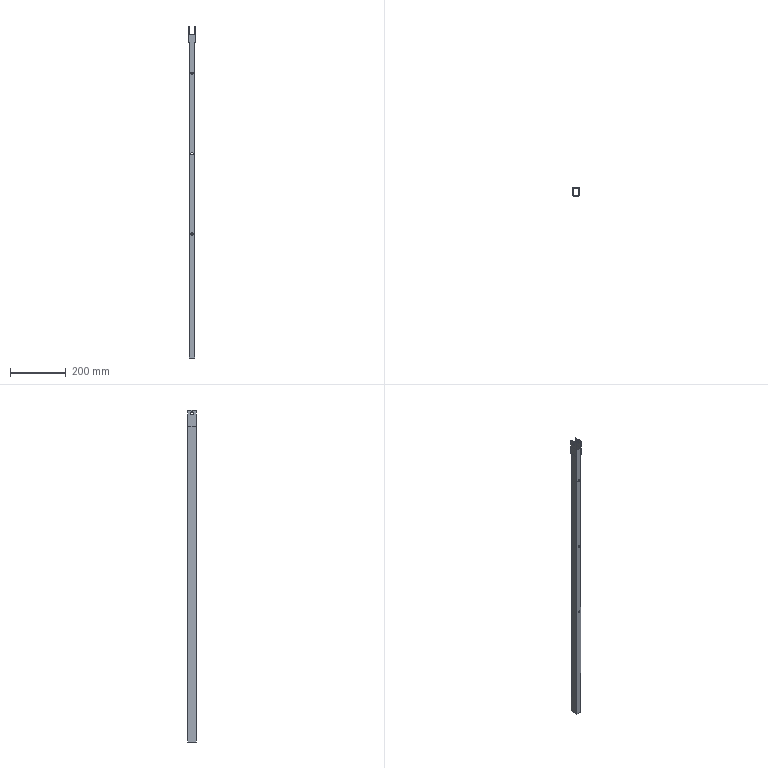Part | SolidWorks | features ICE 4, Extrusion 1, MirrorPattern 1 | 1 solid | 38 faces | box 22 x 30 x 1189 mm | volume 114398 mm3 | cylinder 20 | plane 18 | commonest cylinder face diameters 8 x12 6 x4 10 x4
STEP:
#1=CARTESIAN_POINT('',(10.,-30.,140.));
#2=VERTEX_POINT('',#1);
#3=CARTESIAN_POINT('',(10.,-30.,148.));
#4=VERTEX_POINT('',#3);
#5=CARTESIAN_POINT('',(10.,-30.,144.));
#6=DIRECTION('',(0.,1.,0.));
#7=DIRECTION('',(0.,0.,1.));
#8=AXIS2_PLACEMENT_3D('',#5,#6,#7);
#9=CIRCLE('',#8,4.);
#10=EDGE_CURVE('',#2,#4,#9,.T.);
#11=ORIENTED_EDGE('',*,*,#10,.F.);
#12=CARTESIAN_POINT('',(10.,-29.,140.));
#13=VERTEX_POINT('',#12);
#14=CARTESIAN_POINT('',(10.,-30.,140.));
#15=DIRECTION('',(0.,1.,0.));
#16=VECTOR('',#15,1000.);
#17=LINE('',#14,#16);
#18=EDGE_CURVE('',#2,#13,#17,.T.);
#19=ORIENTED_EDGE('',*,*,#18,.T.);
#20=CARTESIAN_POINT('',(10.,-29.,148.));
#21=VERTEX_POINT('',#20);
#22=CARTESIAN_POINT('',(10.,-29.,144.));
#23=DIRECTION('',(0.,1.,0.));
#24=DIRECTION('',(0.,0.,1.));
#25=AXIS2_PLACEMENT_3D('',#22,#23,#24);
#26=CIRCLE('',#25,4.);
#27=EDGE_CURVE('',#13,#21,#26,.T.);
#28=ORIENTED_EDGE('',*,*,#27,.T.);
#29=CARTESIAN_POINT('',(10.,-30.,148.));
#30=DIRECTION('',(0.,1.,0.));
#31=VECTOR('',#30,1000.);
#32=LINE('',#29,#31);
#33=EDGE_CURVE('',#4,#21,#32,.T.);
#34=ORIENTED_EDGE('',*,*,#33,.F.);
#35=EDGE_LOOP('',(#11,#19,#28,#34));
#36=FACE_OUTER_BOUND('',#35,.T.);
#37=CARTESIAN_POINT('',(10.,-30.,144.));
#38=DIRECTION('',(0.,1.,0.));
#39=DIRECTION('',(0.,0.,1.));
#40=AXIS2_PLACEMENT_3D('',#37,#38,#39);
#41=CYLINDRICAL_SURFACE('',#40,4.);
#42=ADVANCED_FACE('',(#36),#41,.F.);
#43=CARTESIAN_POINT('',(10.,-30.,428.));
#44=VERTEX_POINT('',#43);
#45=CARTESIAN_POINT('',(10.,-30.,436.));
#46=VERTEX_POINT('',#45);
#47=CARTESIAN_POINT('',(10.,-30.,432.));
#48=DIRECTION('',(0.,1.,0.));
#49=DIRECTION('',(0.,0.,1.));
#50=AXIS2_PLACEMENT_3D('',#47,#48,#49);
#51=CIRCLE('',#50,4.);
#52=EDGE_CURVE('',#44,#46,#51,.T.);
#53=ORIENTED_EDGE('',*,*,#52,.F.);
#54=CARTESIAN_POINT('',(10.,-29.,428.));
#55=VERTEX_POINT('',#54);
#56=CARTESIAN_POINT('',(10.,-30.,428.));
#57=DIRECTION('',(0.,1.,0.));
#58=VECTOR('',#57,1000.);
#59=LINE('',#56,#58);
#60=EDGE_CURVE('',#44,#55,#59,.T.);
#61=ORIENTED_EDGE('',*,*,#60,.T.);
#62=CARTESIAN_POINT('',(10.,-29.,436.));
#63=VERTEX_POINT('',#62);
#64=CARTESIAN_POINT('',(10.,-29.,432.));
#65=DIRECTION('',(0.,1.,0.));
#66=DIRECTION('',(0.,0.,1.));
#67=AXIS2_PLACEMENT_3D('',#64,#65,#66);
#68=CIRCLE('',#67,4.);
#69=EDGE_CURVE('',#55,#63,#68,.T.);
#70=ORIENTED_EDGE('',*,*,#69,.T.);
#71=CARTESIAN_POINT('',(10.,-30.,436.));
#72=DIRECTION('',(0.,1.,0.));
#73=VECTOR('',#72,1000.);
#74=LINE('',#71,#73);
#75=EDGE_CURVE('',#46,#63,#74,.T.);
#76=ORIENTED_EDGE('',*,*,#75,.F.);
#77=EDGE_LOOP('',(#53,#61,#70,#76));
#78=FACE_OUTER_BOUND('',#77,.T.);
#79=CARTESIAN_POINT('',(10.,-30.,432.));
#80=DIRECTION('',(0.,1.,0.));
#81=DIRECTION('',(0.,0.,1.));
#82=AXIS2_PLACEMENT_3D('',#79,#80,#81);
#83=CYLINDRICAL_SURFACE('',#82,4.);
#84=ADVANCED_FACE('',(#78),#83,.F.);
#85=CARTESIAN_POINT('',(10.,-30.,716.));
#86=VERTEX_POINT('',#85);
#87=CARTESIAN_POINT('',(10.,-30.,724.));
#88=VERTEX_POINT('',#87);
#89=CARTESIAN_POINT('',(10.,-30.,720.));
#90=DIRECTION('',(0.,1.,0.));
#91=DIRECTION('',(0.,0.,1.));
#92=AXIS2_PLACEMENT_3D('',#89,#90,#91);
#93=CIRCLE('',#92,4.);
#94=EDGE_CURVE('',#86,#88,#93,.T.);
#95=ORIENTED_EDGE('',*,*,#94,.F.);
#96=CARTESIAN_POINT('',(10.,-29.,716.));
#97=VERTEX_POINT('',#96);
#98=CARTESIAN_POINT('',(10.,-30.,716.));
#99=DIRECTION('',(0.,1.,0.));
#100=VECTOR('',#99,1000.);
#101=LINE('',#98,#100);
#102=EDGE_CURVE('',#86,#97,#101,.T.);
#103=ORIENTED_EDGE('',*,*,#102,.T.);
#104=CARTESIAN_POINT('',(10.,-29.,724.));
#105=VERTEX_POINT('',#104);
#106=CARTESIAN_POINT('',(10.,-29.,720.));
#107=DIRECTION('',(0.,1.,0.));
#108=DIRECTION('',(0.,0.,1.));
#109=AXIS2_PLACEMENT_3D('',#106,#107,#108);
#110=CIRCLE('',#109,4.);
#111=EDGE_CURVE('',#97,#105,#110,.T.);
#112=ORIENTED_EDGE('',*,*,#111,.T.);
#113=CARTESIAN_POINT('',(10.,-30.,724.));
#114=DIRECTION('',(0.,1.,0.));
#115=VECTOR('',#114,1000.);
#116=LINE('',#113,#115);
#117=EDGE_CURVE('',#88,#105,#116,.T.);
#118=ORIENTED_EDGE('',*,*,#117,.F.);
#119=EDGE_LOOP('',(#95,#103,#112,#118));
#120=FACE_OUTER_BOUND('',#119,.T.);
#121=CARTESIAN_POINT('',(10.,-30.,720.));
#122=DIRECTION('',(0.,1.,0.));
#123=DIRECTION('',(0.,0.,1.));
#124=AXIS2_PLACEMENT_3D('',#121,#122,#123);
#125=CYLINDRICAL_SURFACE('',#124,4.);
#126=ADVANCED_FACE('',(#120),#125,.F.);
#127=CARTESIAN_POINT('',(10.,-1.,148.));
#128=VERTEX_POINT('',#127);
#129=CARTESIAN_POINT('',(10.,-1.,140.));
#130=VERTEX_POINT('',#129);
#131=CARTESIAN_POINT('',(10.,-1.,144.));
#132=DIRECTION('',(0.,-1.,0.));
#133=DIRECTION('',(0.,0.,-1.));
#134=AXIS2_PLACEMENT_3D('',#131,#132,#133);
#135=CIRCLE('',#134,4.);
#136=EDGE_CURVE('',#128,#130,#135,.T.);
#137=ORIENTED_EDGE('',*,*,#136,.T.);
#138=CARTESIAN_POINT('',(10.,0.,140.));
#139=VERTEX_POINT('',#138);
#140=CARTESIAN_POINT('',(10.,-30.,140.));
#141=DIRECTION('',(0.,1.,0.));
#142=VECTOR('',#141,1000.);
#143=LINE('',#140,#142);
#144=EDGE_CURVE('',#130,#139,#143,.T.);
#145=ORIENTED_EDGE('',*,*,#144,.T.);
#146=CARTESIAN_POINT('',(10.,0.,148.));
#147=VERTEX_POINT('',#146);
#148=CARTESIAN_POINT('',(10.,0.,144.));
#149=DIRECTION('',(0.,1.,0.));
#150=DIRECTION('',(0.,0.,1.));
#151=AXIS2_PLACEMENT_3D('',#148,#149,#150);
#152=CIRCLE('',#151,4.);
#153=EDGE_CURVE('',#139,#147,#152,.T.);
#154=ORIENTED_EDGE('',*,*,#153,.T.);
#155=CARTESIAN_POINT('',(10.,-30.,148.));
#156=DIRECTION('',(0.,1.,0.));
#157=VECTOR('',#156,1000.);
#158=LINE('',#155,#157);
#159=EDGE_CURVE('',#128,#147,#158,.T.);
#160=ORIENTED_EDGE('',*,*,#159,.F.);
#161=EDGE_LOOP('',(#137,#145,#154,#160));
#162=FACE_OUTER_BOUND('',#161,.T.);
#163=CARTESIAN_POINT('',(10.,-30.,144.));
#164=DIRECTION('',(0.,1.,0.));
#165=DIRECTION('',(0.,0.,1.));
#166=AXIS2_PLACEMENT_3D('',#163,#164,#165);
#167=CYLINDRICAL_SURFACE('',#166,4.);
#168=ADVANCED_FACE('',(#162),#167,.F.);
#169=CARTESIAN_POINT('',(10.,-1.,436.));
#170=VERTEX_POINT('',#169);
#171=CARTESIAN_POINT('',(10.,-1.,428.));
#172=VERTEX_POINT('',#171);
#173=CARTESIAN_POINT('',(10.,-1.,432.));
#174=DIRECTION('',(0.,-1.,0.));
#175=DIRECTION('',(0.,0.,-1.));
#176=AXIS2_PLACEMENT_3D('',#173,#174,#175);
#177=CIRCLE('',#176,4.);
#178=EDGE_CURVE('',#170,#172,#177,.T.);
#179=ORIENTED_EDGE('',*,*,#178,.T.);
#180=CARTESIAN_POINT('',(10.,0.,428.));
#181=VERTEX_POINT('',#180);
#182=CARTESIAN_POINT('',(10.,-30.,428.));
#183=DIRECTION('',(0.,1.,0.));
#184=VECTOR('',#183,1000.);
#185=LINE('',#182,#184);
#186=EDGE_CURVE('',#172,#181,#185,.T.);
#187=ORIENTED_EDGE('',*,*,#186,.T.);
#188=CARTESIAN_POINT('',(10.,0.,436.));
#189=VERTEX_POINT('',#188);
#190=CARTESIAN_POINT('',(10.,0.,432.));
#191=DIRECTION('',(0.,1.,0.));
#192=DIRECTION('',(0.,0.,1.));
#193=AXIS2_PLACEMENT_3D('',#190,#191,#192);
#194=CIRCLE('',#193,4.);
#195=EDGE_CURVE('',#181,#189,#194,.T.);
#196=ORIENTED_EDGE('',*,*,#195,.T.);
#197=CARTESIAN_POINT('',(10.,-30.,436.));
#198=DIRECTION('',(0.,1.,0.));
#199=VECTOR('',#198,1000.);
#200=LINE('',#197,#199);
#201=EDGE_CURVE('',#170,#189,#200,.T.);
#202=ORIENTED_EDGE('',*,*,#201,.F.);
#203=EDGE_LOOP('',(#179,#187,#196,#202));
#204=FACE_OUTER_BOUND('',#203,.T.);
#205=CARTESIAN_POINT('',(10.,-30.,432.));
#206=DIRECTION('',(0.,1.,0.));
#207=DIRECTION('',(0.,0.,1.));
#208=AXIS2_PLACEMENT_3D('',#205,#206,#207);
#209=CYLINDRICAL_SURFACE('',#208,4.);
#210=ADVANCED_FACE('',(#204),#209,.F.);
#211=CARTESIAN_POINT('',(10.,-1.,724.));
#212=VERTEX_POINT('',#211);
#213=CARTESIAN_POINT('',(10.,-1.,716.));
#214=VERTEX_POINT('',#213);
#215=CARTESIAN_POINT('',(10.,-1.,720.));
#216=DIRECTION('',(0.,-1.,0.));
#217=DIRECTION('',(0.,0.,-1.));
#218=AXIS2_PLACEMENT_3D('',#215,#216,#217);
#219=CIRCLE('',#218,4.);
#220=EDGE_CURVE('',#212,#214,#219,.T.);
#221=ORIENTED_EDGE('',*,*,#220,.T.);
#222=CARTESIAN_POINT('',(10.,0.,716.));
#223=VERTEX_POINT('',#222);
#224=CARTESIAN_POINT('',(10.,-30.,716.));
#225=DIRECTION('',(0.,1.,0.));
#226=VECTOR('',#225,1000.);
#227=LINE('',#224,#226);
#228=EDGE_CURVE('',#214,#223,#227,.T.);
#229=ORIENTED_EDGE('',*,*,#228,.T.);
#230=CARTESIAN_POINT('',(10.,0.,724.));
#231=VERTEX_POINT('',#230);
#232=CARTESIAN_POINT('',(10.,0.,720.));
#233=DIRECTION('',(0.,1.,0.));
#234=DIRECTION('',(0.,0.,1.));
#235=AXIS2_PLACEMENT_3D('',#232,#233,#234);
#236=CIRCLE('',#235,4.);
#237=EDGE_CURVE('',#223,#231,#236,.T.);
#238=ORIENTED_EDGE('',*,*,#237,.T.);
#239=CARTESIAN_POINT('',(10.,-30.,724.));
#240=DIRECTION('',(0.,1.,0.));
#241=VECTOR('',#240,1000.);
#242=LINE('',#239,#241);
#243=EDGE_CURVE('',#212,#231,#242,.T.);
#244=ORIENTED_EDGE('',*,*,#243,.F.);
#245=EDGE_LOOP('',(#221,#229,#238,#244));
#246=FACE_OUTER_BOUND('',#245,.T.);
#247=CARTESIAN_POINT('',(10.,-30.,720.));
#248=DIRECTION('',(0.,1.,0.));
#249=DIRECTION('',(0.,0.,1.));
#250=AXIS2_PLACEMENT_3D('',#247,#248,#249);
#251=CYLINDRICAL_SURFACE('',#250,4.);
#252=ADVANCED_FACE('',(#246),#251,.F.);
#253=CARTESIAN_POINT('',(-1.,-20.,877.5));
#254=VERTEX_POINT('',#253);
#255=CARTESIAN_POINT('',(-1.,-10.,877.5));
#256=VERTEX_POINT('',#255);
#257=CARTESIAN_POINT('',(-1.,-15.,877.5));
#258=DIRECTION('',(1.,0.,0.));
#259=DIRECTION('',(0.,1.,0.));
#260=AXIS2_PLACEMENT_3D('',#257,#258,#259);
#261=CIRCLE('',#260,5.);
#262=EDGE_CURVE('',#254,#256,#261,.T.);
#263=ORIENTED_EDGE('',*,*,#262,.F.);
#264=CARTESIAN_POINT('',(0.,-20.,877.5));
#265=VERTEX_POINT('',#264);
#266=CARTESIAN_POINT('',(-1.,-20.,877.5));
#267=DIRECTION('',(1.,0.,0.));
#268=VECTOR('',#267,1000.);
#269=LINE('',#266,#268);
#270=EDGE_CURVE('',#254,#265,#269,.T.);
#271=ORIENTED_EDGE('',*,*,#270,.T.);
#272=CARTESIAN_POINT('',(0.,-10.,877.5));
#273=VERTEX_POINT('',#272);
#274=CARTESIAN_POINT('',(0.,-15.,877.5));
#275=DIRECTION('',(-1.,0.,0.));
#276=DIRECTION('',(0.,-1.,0.));
#277=AXIS2_PLACEMENT_3D('',#274,#275,#276);
#278=CIRCLE('',#277,5.);
#279=EDGE_CURVE('',#273,#265,#278,.T.);
#280=ORIENTED_EDGE('',*,*,#279,.F.);
#281=CARTESIAN_POINT('',(-1.,-10.,877.5));
#282=DIRECTION('',(1.,0.,0.));
#283=VECTOR('',#282,1000.);
#284=LINE('',#281,#283);
#285=EDGE_CURVE('',#256,#273,#284,.T.);
#286=ORIENTED_EDGE('',*,*,#285,.F.);
#287=EDGE_LOOP('',(#263,#271,#280,#286));
#288=FACE_OUTER_BOUND('',#287,.T.);
#289=CARTESIAN_POINT('',(-1.,-15.,877.5));
#290=DIRECTION('',(1.,0.,0.));
#291=DIRECTION('',(0.,1.,0.));
#292=AXIS2_PLACEMENT_3D('',#289,#290,#291);
#293=CYLINDRICAL_SURFACE('',#292,5.);
#294=ADVANCED_FACE('',(#288),#293,.F.);
#295=CARTESIAN_POINT('',(20.,-20.,877.5));
#296=VERTEX_POINT('',#295);
#297=CARTESIAN_POINT('',(20.,-10.,877.5));
#298=VERTEX_POINT('',#297);
#299=CARTESIAN_POINT('',(20.,-15.,877.5));
#300=DIRECTION('',(1.,0.,0.));
#301=DIRECTION('',(0.,1.,0.));
#302=AXIS2_PLACEMENT_3D('',#299,#300,#301);
#303=CIRCLE('',#302,5.);
#304=EDGE_CURVE('',#296,#298,#303,.T.);
#305=ORIENTED_EDGE('',*,*,#304,.F.);
#306=CARTESIAN_POINT('',(21.,-20.,877.5));
#307=VERTEX_POINT('',#306);
#308=CARTESIAN_POINT('',(-1.,-20.,877.5));
#309=DIRECTION('',(1.,0.,0.));
#310=VECTOR('',#309,1000.);
#311=LINE('',#308,#310);
#312=EDGE_CURVE('',#296,#307,#311,.T.);
#313=ORIENTED_EDGE('',*,*,#312,.T.);
#314=CARTESIAN_POINT('',(21.,-10.,877.5));
#315=VERTEX_POINT('',#314);
#316=CARTESIAN_POINT('',(21.,-15.,877.5));
#317=DIRECTION('',(1.,0.,0.));
#318=DIRECTION('',(0.,1.,0.));
#319=AXIS2_PLACEMENT_3D('',#316,#317,#318);
#320=CIRCLE('',#319,5.);
#321=EDGE_CURVE('',#307,#315,#320,.T.);
#322=ORIENTED_EDGE('',*,*,#321,.T.);
#323=CARTESIAN_POINT('',(-1.,-10.,877.5));
#324=DIRECTION('',(1.,0.,0.));
#325=VECTOR('',#324,1000.);
#326=LINE('',#323,#325);
#327=EDGE_CURVE('',#298,#315,#326,.T.);
#328=ORIENTED_EDGE('',*,*,#327,.F.);
#329=EDGE_LOOP('',(#305,#313,#322,#328));
#330=FACE_OUTER_BOUND('',#329,.T.);
#331=CARTESIAN_POINT('',(-1.,-15.,877.5));
#332=DIRECTION('',(1.,0.,0.));
#333=DIRECTION('',(0.,1.,0.));
#334=AXIS2_PLACEMENT_3D('',#331,#332,#333);
#335=CYLINDRICAL_SURFACE('',#334,5.);
#336=ADVANCED_FACE('',(#330),#335,.F.);
#337=CARTESIAN_POINT('',(0.,0.,829.));
#338=VERTEX_POINT('',#337);
#339=CARTESIAN_POINT('',(0.,-30.,829.));
#340=VERTEX_POINT('',#339);
#341=CARTESIAN_POINT('',(0.,-30.,829.));
#342=DIRECTION('',(0.,-1.,0.));
#343=VECTOR('',#342,1000.);
#344=LINE('',#341,#343);
#345=EDGE_CURVE('',#338,#340,#344,.T.);
#346=ORIENTED_EDGE('',*,*,#345,.F.);
#347=CARTESIAN_POINT('',(0.,0.,-300.));
#348=VERTEX_POINT('',#347);
#349=CARTESIAN_POINT('',(0.,0.,859.));
#350=DIRECTION('',(0.,0.,-1.));
#351=VECTOR('',#350,1000.);
#352=LINE('',#349,#351);
#353=EDGE_CURVE('',#338,#348,#352,.T.);
#354=ORIENTED_EDGE('',*,*,#353,.T.);
#355=CARTESIAN_POINT('',(0.,-30.,-300.));
#356=VERTEX_POINT('',#355);
#357=CARTESIAN_POINT('',(0.,-30.,-300.));
#358=DIRECTION('',(0.,1.,0.));
#359=VECTOR('',#358,1000.);
#360=LINE('',#357,#359);
#361=EDGE_CURVE('',#356,#348,#360,.T.);
#362=ORIENTED_EDGE('',*,*,#361,.F.);
#363=CARTESIAN_POINT('',(0.,-30.,859.));
#364=DIRECTION('',(0.,0.,-1.));
#365=VECTOR('',#364,1000.);
#366=LINE('',#363,#365);
#367=EDGE_CURVE('',#340,#356,#366,.T.);
#368=ORIENTED_EDGE('',*,*,#367,.F.);
#369=EDGE_LOOP('',(#346,#354,#362,#368));
#370=FACE_OUTER_BOUND('',#369,.T.);
#371=CARTESIAN_POINT('',(0.,0.,859.));
#372=DIRECTION('',(1.,0.,0.));
#373=DIRECTION('',(0.,1.,0.));
#374=AXIS2_PLACEMENT_3D('',#371,#372,#373);
#375=PLANE('',#374);
#376=ADVANCED_FACE('',(#370),#375,.F.);
#377=CARTESIAN_POINT('',(0.,0.,859.));
#378=VERTEX_POINT('',#377);
#379=CARTESIAN_POINT('',(0.,-30.,859.));
#380=VERTEX_POINT('',#379);
#381=CARTESIAN_POINT('',(0.,0.,859.));
#382=DIRECTION('',(0.,-1.,0.));
#383=VECTOR('',#382,1000.);
#384=LINE('',#381,#383);
#385=EDGE_CURVE('',#378,#380,#384,.T.);
#386=ORIENTED_EDGE('',*,*,#385,.T.);
#387=CARTESIAN_POINT('',(20.,-30.,859.));
#388=VERTEX_POINT('',#387);
#389=CARTESIAN_POINT('',(0.,-30.,859.));
#390=DIRECTION('',(1.,0.,0.));
#391=VECTOR('',#390,1000.);
#392=LINE('',#389,#391);
#393=EDGE_CURVE('',#380,#388,#392,.T.);
#394=ORIENTED_EDGE('',*,*,#393,.T.);
#395=CARTESIAN_POINT('',(20.,0.,859.));
#396=VERTEX_POINT('',#395);
#397=CARTESIAN_POINT('',(20.,0.,859.));
#398=DIRECTION('',(0.,1.,0.));
#399=VECTOR('',#398,1000.);
#400=LINE('',#397,#399);
#401=EDGE_CURVE('',#388,#396,#400,.T.);
#402=ORIENTED_EDGE('',*,*,#401,.T.);
#403=CARTESIAN_POINT('',(0.,0.,859.));
#404=DIRECTION('',(-1.,0.,0.));
#405=VECTOR('',#404,1000.);
#406=LINE('',#403,#405);
#407=EDGE_CURVE('',#396,#378,#406,.T.);
#408=ORIENTED_EDGE('',*,*,#407,.T.);
#409=EDGE_LOOP('',(#386,#394,#402,#408));
#410=FACE_OUTER_BOUND('',#409,.T.);
#411=CARTESIAN_POINT('',(1.,-29.,859.));
#412=VERTEX_POINT('',#411);
#413=CARTESIAN_POINT('',(19.,-29.,859.));
#414=VERTEX_POINT('',#413);
#415=CARTESIAN_POINT('',(1.,-29.,859.));
#416=DIRECTION('',(1.,0.,0.));
#417=VECTOR('',#416,1000.);
#418=LINE('',#415,#417);
#419=EDGE_CURVE('',#412,#414,#418,.T.);
#420=ORIENTED_EDGE('',*,*,#419,.F.);
#421=CARTESIAN_POINT('',(1.,-1.,859.));
#422=VERTEX_POINT('',#421);
#423=CARTESIAN_POINT('',(1.,-1.,859.));
#424=DIRECTION('',(0.,-1.,0.));
#425=VECTOR('',#424,1000.);
#426=LINE('',#423,#425);
#427=EDGE_CURVE('',#422,#412,#426,.T.);
#428=ORIENTED_EDGE('',*,*,#427,.F.);
#429=CARTESIAN_POINT('',(19.,-1.,859.));
#430=VERTEX_POINT('',#429);
#431=CARTESIAN_POINT('',(1.,-1.,859.));
#432=DIRECTION('',(-1.,0.,0.));
#433=VECTOR('',#432,1000.);
#434=LINE('',#431,#433);
#435=EDGE_CURVE('',#430,#422,#434,.T.);
#436=ORIENTED_EDGE('',*,*,#435,.F.);
#437=CARTESIAN_POINT('',(19.,-1.,859.));
#438=DIRECTION('',(0.,1.,0.));
#439=VECTOR('',#438,1000.);
#440=LINE('',#437,#439);
#441=EDGE_CURVE('',#414,#430,#440,.T.);
#442=ORIENTED_EDGE('',*,*,#441,.F.);
#443=EDGE_LOOP('',(#420,#428,#436,#442));
#444=FACE_BOUND('',#443,.T.);
#445=CARTESIAN_POINT('',(0.,0.,859.));
#446=DIRECTION('',(0.,0.,1.));
#447=DIRECTION('',(1.,0.,0.));
#448=AXIS2_PLACEMENT_3D('',#445,#446,#447);
#449=PLANE('',#448);
#450=ADVANCED_FACE('',(#410,#444),#449,.T.);
#451=CARTESIAN_POINT('',(10.,-30.,144.));
#452=DIRECTION('',(0.,1.,0.));
#453=DIRECTION('',(0.,0.,1.));
#454=AXIS2_PLACEMENT_3D('',#451,#452,#453);
#455=CIRCLE('',#454,4.);
#456=EDGE_CURVE('',#4,#2,#455,.T.);
#457=ORIENTED_EDGE('',*,*,#456,.T.);
#458=ORIENTED_EDGE('',*,*,#10,.T.);
#459=EDGE_LOOP('',(#457,#458));
#460=FACE_BOUND('',#459,.T.);
#461=CARTESIAN_POINT('',(10.,-30.,432.));
#462=DIRECTION('',(0.,1.,0.));
#463=DIRECTION('',(0.,0.,1.));
#464=AXIS2_PLACEMENT_3D('',#461,#462,#463);
#465=CIRCLE('',#464,4.);
#466=EDGE_CURVE('',#46,#44,#465,.T.);
#467=ORIENTED_EDGE('',*,*,#466,.T.);
#468=ORIENTED_EDGE('',*,*,#52,.T.);
#469=EDGE_LOOP('',(#467,#468));
#470=FACE_BOUND('',#469,.T.);
#471=CARTESIAN_POINT('',(10.,-30.,720.));
#472=DIRECTION('',(0.,1.,0.));
#473=DIRECTION('',(0.,0.,1.));
#474=AXIS2_PLACEMENT_3D('',#471,#472,#473);
#475=CIRCLE('',#474,4.);
#476=EDGE_CURVE('',#88,#86,#475,.T.);
#477=ORIENTED_EDGE('',*,*,#476,.T.);
#478=ORIENTED_EDGE('',*,*,#94,.T.);
#479=EDGE_LOOP('',(#477,#478));
#480=FACE_BOUND('',#479,.T.);
#481=ORIENTED_EDGE('',*,*,#367,.T.);
#482=CARTESIAN_POINT('',(20.,-30.,-300.));
#483=VERTEX_POINT('',#482);
#484=CARTESIAN_POINT('',(20.,-30.,-300.));
#485=DIRECTION('',(-1.,0.,0.));
#486=VECTOR('',#485,1000.);
#487=LINE('',#484,#486);
#488=EDGE_CURVE('',#483,#356,#487,.T.);
#489=ORIENTED_EDGE('',*,*,#488,.F.);
#490=CARTESIAN_POINT('',(20.,-30.,829.));
#491=VERTEX_POINT('',#490);
#492=CARTESIAN_POINT('',(20.,-30.,859.));
#493=DIRECTION('',(0.,0.,-1.));
#494=VECTOR('',#493,1000.);
#495=LINE('',#492,#494);
#496=EDGE_CURVE('',#491,#483,#495,.T.);
#497=ORIENTED_EDGE('',*,*,#496,.F.);
#498=CARTESIAN_POINT('',(21.,-30.,829.));
#499=VERTEX_POINT('',#498);
#500=CARTESIAN_POINT('',(21.,-30.,829.));
#501=DIRECTION('',(-1.,0.,0.));
#502=VECTOR('',#501,1000.);
#503=LINE('',#500,#502);
#504=EDGE_CURVE('',#499,#491,#503,.T.);
#505=ORIENTED_EDGE('',*,*,#504,.F.);
#506=CARTESIAN_POINT('',(21.,-30.,886.));
#507=VERTEX_POINT('',#506);
#508=CARTESIAN_POINT('',(21.,-30.,859.));
#509=DIRECTION('',(0.,0.,1.));
#510=VECTOR('',#509,1000.);
#511=LINE('',#508,#510);
#512=EDGE_CURVE('',#499,#507,#511,.T.);
#513=ORIENTED_EDGE('',*,*,#512,.T.);
#514=CARTESIAN_POINT('',(20.,-30.,886.));
#515=VERTEX_POINT('',#514);
#516=CARTESIAN_POINT('',(21.,-30.,886.));
#517=DIRECTION('',(-1.,0.,0.));
#518=VECTOR('',#517,1000.);
#519=LINE('',#516,#518);
#520=EDGE_CURVE('',#507,#515,#519,.T.);
#521=ORIENTED_EDGE('',*,*,#520,.T.);
#522=CARTESIAN_POINT('',(20.,-30.,829.));
#523=DIRECTION('',(0.,0.,1.));
#524=VECTOR('',#523,1000.);
#525=LINE('',#522,#524);
#526=EDGE_CURVE('',#388,#515,#525,.T.);
#527=ORIENTED_EDGE('',*,*,#526,.F.);
#528=ORIENTED_EDGE('',*,*,#393,.F.);
#529=CARTESIAN_POINT('',(0.,-30.,886.));
#530=VERTEX_POINT('',#529);
#531=CARTESIAN_POINT('',(0.,-30.,859.));
#532=DIRECTION('',(0.,0.,1.));
#533=VECTOR('',#532,1000.);
#534=LINE('',#531,#533);
#535=EDGE_CURVE('',#380,#530,#534,.T.);
#536=ORIENTED_EDGE('',*,*,#535,.T.);
#537=CARTESIAN_POINT('',(-1.,-30.,886.));
#538=VERTEX_POINT('',#537);
#539=CARTESIAN_POINT('',(-1.,-30.,886.));
#540=DIRECTION('',(1.,0.,0.));
#541=VECTOR('',#540,1000.);
#542=LINE('',#539,#541);
#543=EDGE_CURVE('',#538,#530,#542,.T.);
#544=ORIENTED_EDGE('',*,*,#543,.F.);
#545=CARTESIAN_POINT('',(-1.,-30.,829.));
#546=VERTEX_POINT('',#545);
#547=CARTESIAN_POINT('',(-1.,-30.,829.));
#548=DIRECTION('',(0.,0.,1.));
#549=VECTOR('',#548,1000.);
#550=LINE('',#547,#549);
#551=EDGE_CURVE('',#546,#538,#550,.T.);
#552=ORIENTED_EDGE('',*,*,#551,.F.);
#553=CARTESIAN_POINT('',(-1.,-30.,829.));
#554=DIRECTION('',(1.,0.,0.));
#555=VECTOR('',#554,1000.);
#556=LINE('',#553,#555);
#557=EDGE_CURVE('',#546,#340,#556,.T.);
#558=ORIENTED_EDGE('',*,*,#557,.T.);
#559=EDGE_LOOP('',(#481,#489,#497,#505,#513,#521,#527,#528,#536,#544,#552,#558));
#560=FACE_OUTER_BOUND('',#559,.T.);
#561=CARTESIAN_POINT('',(0.,-30.,859.));
#562=DIRECTION('',(0.,1.,0.));
#563=DIRECTION('',(0.,0.,1.));
#564=AXIS2_PLACEMENT_3D('',#561,#562,#563);
#565=PLANE('',#564);
#566=ADVANCED_FACE('',(#460,#470,#480,#560),#565,.F.);
#567=CARTESIAN_POINT('',(20.,0.,829.));
#568=VERTEX_POINT('',#567);
#569=CARTESIAN_POINT('',(20.,0.,-300.));
#570=VERTEX_POINT('',#569);
#571=CARTESIAN_POINT('',(20.,0.,859.));
#572=DIRECTION('',(0.,0.,-1.));
#573=VECTOR('',#572,1000.);
#574=LINE('',#571,#573);
#575=EDGE_CURVE('',#568,#570,#574,.T.);
#576=ORIENTED_EDGE('',*,*,#575,.F.);
#577=CARTESIAN_POINT('',(20.,-30.,829.));
#578=DIRECTION('',(0.,-1.,0.));
#579=VECTOR('',#578,1000.);
#580=LINE('',#577,#579);
#581=EDGE_CURVE('',#568,#491,#580,.T.);
#582=ORIENTED_EDGE('',*,*,#581,.T.);
#583=ORIENTED_EDGE('',*,*,#496,.T.);
#584=CARTESIAN_POINT('',(20.,0.,-300.));
#585=DIRECTION('',(0.,-1.,0.));
#586=VECTOR('',#585,1000.);
#587=LINE('',#584,#586);
#588=EDGE_CURVE('',#570,#483,#587,.T.);
#589=ORIENTED_EDGE('',*,*,#588,.F.);
#590=EDGE_LOOP('',(#576,#582,#583,#589));
#591=FACE_OUTER_BOUND('',#590,.T.);
#592=CARTESIAN_POINT('',(20.,0.,859.));
#593=DIRECTION('',(-1.,0.,0.));
#594=DIRECTION('',(0.,-1.,0.));
#595=AXIS2_PLACEMENT_3D('',#592,#593,#594);
#596=PLANE('',#595);
#597=ADVANCED_FACE('',(#591),#596,.F.);
#598=CARTESIAN_POINT('',(10.,0.,144.));
#599=DIRECTION('',(0.,1.,0.));
#600=DIRECTION('',(0.,0.,1.));
#601=AXIS2_PLACEMENT_3D('',#598,#599,#600);
#602=CIRCLE('',#601,4.);
#603=EDGE_CURVE('',#147,#139,#602,.T.);
#604=ORIENTED_EDGE('',*,*,#603,.F.);
#605=ORIENTED_EDGE('',*,*,#153,.F.);
#606=EDGE_LOOP('',(#604,#605));
#607=FACE_BOUND('',#606,.T.);
#608=CARTESIAN_POINT('',(10.,0.,432.));
#609=DIRECTION('',(0.,1.,0.));
#610=DIRECTION('',(0.,0.,1.));
#611=AXIS2_PLACEMENT_3D('',#608,#609,#610);
#612=CIRCLE('',#611,4.);
#613=EDGE_CURVE('',#189,#181,#612,.T.);
#614=ORIENTED_EDGE('',*,*,#613,.F.);
#615=ORIENTED_EDGE('',*,*,#195,.F.);
#616=EDGE_LOOP('',(#614,#615));
#617=FACE_BOUND('',#616,.T.);
#618=CARTESIAN_POINT('',(10.,0.,720.));
#619=DIRECTION('',(0.,1.,0.));
#620=DIRECTION('',(0.,0.,1.));
#621=AXIS2_PLACEMENT_3D('',#618,#619,#620);
#622=CIRCLE('',#621,4.);
#623=EDGE_CURVE('',#231,#223,#622,.T.);
#624=ORIENTED_EDGE('',*,*,#623,.F.);
#625=ORIENTED_EDGE('',*,*,#237,.F.);
#626=EDGE_LOOP('',(#624,#625));
#627=FACE_BOUND('',#626,.T.);
#628=ORIENTED_EDGE('',*,*,#575,.T.);
#629=CARTESIAN_POINT('',(0.,0.,-300.));
#630=DIRECTION('',(1.,0.,0.));
#631=VECTOR('',#630,1000.);
#632=LINE('',#629,#631);
#633=EDGE_CURVE('',#348,#570,#632,.T.);
#634=ORIENTED_EDGE('',*,*,#633,.F.);
#635=ORIENTED_EDGE('',*,*,#353,.F.);
#636=CARTESIAN_POINT('',(-1.,0.,829.));
#637=VERTEX_POINT('',#636);
#638=CARTESIAN_POINT('',(-1.,0.,829.));
#639=DIRECTION('',(1.,0.,0.));
#640=VECTOR('',#639,1000.);
#641=LINE('',#638,#640);
#642=EDGE_CURVE('',#637,#338,#641,.T.);
#643=ORIENTED_EDGE('',*,*,#642,.F.);
#644=CARTESIAN_POINT('',(-1.,0.,886.));
#645=VERTEX_POINT('',#644);
#646=CARTESIAN_POINT('',(-1.,0.,886.));
#647=DIRECTION('',(0.,0.,-1.));
#648=VECTOR('',#647,1000.);
#649=LINE('',#646,#648);
#650=EDGE_CURVE('',#645,#637,#649,.T.);
#651=ORIENTED_EDGE('',*,*,#650,.F.);
#652=CARTESIAN_POINT('',(0.,0.,886.));
#653=VERTEX_POINT('',#652);
#654=CARTESIAN_POINT('',(-1.,0.,886.));
#655=DIRECTION('',(1.,0.,0.));
#656=VECTOR('',#655,1000.);
#657=LINE('',#654,#656);
#658=EDGE_CURVE('',#645,#653,#657,.T.);
#659=ORIENTED_EDGE('',*,*,#658,.T.);
#660=CARTESIAN_POINT('',(0.,0.,859.));
#661=DIRECTION('',(0.,0.,-1.));
#662=VECTOR('',#661,1000.);
#663=LINE('',#660,#662);
#664=EDGE_CURVE('',#653,#378,#663,.T.);
#665=ORIENTED_EDGE('',*,*,#664,.T.);
#666=ORIENTED_EDGE('',*,*,#407,.F.);
#667=CARTESIAN_POINT('',(20.,0.,886.));
#668=VERTEX_POINT('',#667);
#669=CARTESIAN_POINT('',(20.,0.,886.));
#670=DIRECTION('',(0.,0.,-1.));
#671=VECTOR('',#670,1000.);
#672=LINE('',#669,#671);
#673=EDGE_CURVE('',#668,#396,#672,.T.);
#674=ORIENTED_EDGE('',*,*,#673,.F.);
#675=CARTESIAN_POINT('',(21.,0.,886.));
#676=VERTEX_POINT('',#675);
#677=CARTESIAN_POINT('',(21.,0.,886.));
#678=DIRECTION('',(-1.,0.,0.));
#679=VECTOR('',#678,1000.);
#680=LINE('',#677,#679);
#681=EDGE_CURVE('',#676,#668,#680,.T.);
#682=ORIENTED_EDGE('',*,*,#681,.F.);
#683=CARTESIAN_POINT('',(21.,0.,829.));
#684=VERTEX_POINT('',#683);
#685=CARTESIAN_POINT('',(21.,0.,859.));
#686=DIRECTION('',(0.,0.,-1.));
#687=VECTOR('',#686,1000.);
#688=LINE('',#685,#687);
#689=EDGE_CURVE('',#676,#684,#688,.T.);
#690=ORIENTED_EDGE('',*,*,#689,.T.);
#691=CARTESIAN_POINT('',(21.,0.,829.));
#692=DIRECTION('',(-1.,0.,0.));
#693=VECTOR('',#692,1000.);
#694=LINE('',#691,#693);
#695=EDGE_CURVE('',#684,#568,#694,.T.);
#696=ORIENTED_EDGE('',*,*,#695,.T.);
#697=EDGE_LOOP('',(#628,#634,#635,#643,#651,#659,#665,#666,#674,#682,#690,#696));
#698=FACE_OUTER_BOUND('',#697,.T.);
#699=CARTESIAN_POINT('',(0.,0.,859.));
#700=DIRECTION('',(0.,-1.,0.));
#701=DIRECTION('',(0.,0.,-1.));
#702=AXIS2_PLACEMENT_3D('',#699,#700,#701);
#703=PLANE('',#702);
#704=ADVANCED_FACE('',(#607,#617,#627,#698),#703,.F.);
#705=CARTESIAN_POINT('',(1.,-29.,-300.));
#706=VERTEX_POINT('',#705);
#707=CARTESIAN_POINT('',(1.,-29.,859.));
#708=DIRECTION('',(0.,0.,-1.));
#709=VECTOR('',#708,1000.);
#710=LINE('',#707,#709);
#711=EDGE_CURVE('',#412,#706,#710,.T.);
#712=ORIENTED_EDGE('',*,*,#711,.T.);
#713=CARTESIAN_POINT('',(1.,-1.,-300.));
#714=VERTEX_POINT('',#713);
#715=CARTESIAN_POINT('',(1.,-1.,-300.));
#716=DIRECTION('',(0.,1.,0.));
#717=VECTOR('',#716,1000.);
#718=LINE('',#715,#717);
#719=EDGE_CURVE('',#706,#714,#718,.T.);
#720=ORIENTED_EDGE('',*,*,#719,.T.);
#721=CARTESIAN_POINT('',(1.,-1.,859.));
#722=DIRECTION('',(0.,0.,-1.));
#723=VECTOR('',#722,1000.);
#724=LINE('',#721,#723);
#725=EDGE_CURVE('',#422,#714,#724,.T.);
#726=ORIENTED_EDGE('',*,*,#725,.F.);
#727=ORIENTED_EDGE('',*,*,#427,.T.);
#728=EDGE_LOOP('',(#712,#720,#726,#727));
#729=FACE_OUTER_BOUND('',#728,.T.);
#730=CARTESIAN_POINT('',(1.,-1.,859.));
#731=DIRECTION('',(1.,0.,0.));
#732=DIRECTION('',(0.,1.,0.));
#733=AXIS2_PLACEMENT_3D('',#730,#731,#732);
#734=PLANE('',#733);
#735=ADVANCED_FACE('',(#729),#734,.T.);
#736=CARTESIAN_POINT('',(10.,-29.,144.));
#737=DIRECTION('',(0.,1.,0.));
#738=DIRECTION('',(0.,0.,1.));
#739=AXIS2_PLACEMENT_3D('',#736,#737,#738);
#740=CIRCLE('',#739,4.);
#741=EDGE_CURVE('',#21,#13,#740,.T.);
#742=ORIENTED_EDGE('',*,*,#741,.F.);
#743=ORIENTED_EDGE('',*,*,#27,.F.);
#744=EDGE_LOOP('',(#742,#743));
#745=FACE_BOUND('',#744,.T.);
#746=CARTESIAN_POINT('',(10.,-29.,432.));
#747=DIRECTION('',(0.,1.,0.));
#748=DIRECTION('',(0.,0.,1.));
#749=AXIS2_PLACEMENT_3D('',#746,#747,#748);
#750=CIRCLE('',#749,4.);
#751=EDGE_CURVE('',#63,#55,#750,.T.);
#752=ORIENTED_EDGE('',*,*,#751,.F.);
#753=ORIENTED_EDGE('',*,*,#69,.F.);
#754=EDGE_LOOP('',(#752,#753));
#755=FACE_BOUND('',#754,.T.);
#756=CARTESIAN_POINT('',(10.,-29.,720.));
#757=DIRECTION('',(0.,1.,0.));
#758=DIRECTION('',(0.,0.,1.));
#759=AXIS2_PLACEMENT_3D('',#756,#757,#758);
#760=CIRCLE('',#759,4.);
#761=EDGE_CURVE('',#105,#97,#760,.T.);
#762=ORIENTED_EDGE('',*,*,#761,.F.);
#763=ORIENTED_EDGE('',*,*,#111,.F.);
#764=EDGE_LOOP('',(#762,#763));
#765=FACE_BOUND('',#764,.T.);
#766=CARTESIAN_POINT('',(19.,-29.,-300.));
#767=VERTEX_POINT('',#766);
#768=CARTESIAN_POINT('',(19.,-29.,859.));
#769=DIRECTION('',(0.,0.,-1.));
#770=VECTOR('',#769,1000.);
#771=LINE('',#768,#770);
#772=EDGE_CURVE('',#414,#767,#771,.T.);
#773=ORIENTED_EDGE('',*,*,#772,.T.);
#774=CARTESIAN_POINT('',(1.,-29.,-300.));
#775=DIRECTION('',(-1.,0.,0.));
#776=VECTOR('',#775,1000.);
#777=LINE('',#774,#776);
#778=EDGE_CURVE('',#767,#706,#777,.T.);
#779=ORIENTED_EDGE('',*,*,#778,.T.);
#780=ORIENTED_EDGE('',*,*,#711,.F.);
#781=ORIENTED_EDGE('',*,*,#419,.T.);
#782=EDGE_LOOP('',(#773,#779,#780,#781));
#783=FACE_OUTER_BOUND('',#782,.T.);
#784=CARTESIAN_POINT('',(1.,-29.,859.));
#785=DIRECTION('',(0.,1.,0.));
#786=DIRECTION('',(0.,0.,1.));
#787=AXIS2_PLACEMENT_3D('',#784,#785,#786);
#788=PLANE('',#787);
#789=ADVANCED_FACE('',(#745,#755,#765,#783),#788,.T.);
#790=CARTESIAN_POINT('',(19.,-1.,-300.));
#791=VERTEX_POINT('',#790);
#792=CARTESIAN_POINT('',(19.,-1.,859.));
#793=DIRECTION('',(0.,0.,-1.));
#794=VECTOR('',#793,1000.);
#795=LINE('',#792,#794);
#796=EDGE_CURVE('',#430,#791,#795,.T.);
#797=ORIENTED_EDGE('',*,*,#796,.T.);
#798=CARTESIAN_POINT('',(19.,-29.,-300.));
#799=DIRECTION('',(0.,-1.,0.));
#800=VECTOR('',#799,1000.);
#801=LINE('',#798,#800);
#802=EDGE_CURVE('',#791,#767,#801,.T.);
#803=ORIENTED_EDGE('',*,*,#802,.T.);
#804=ORIENTED_EDGE('',*,*,#772,.F.);
#805=ORIENTED_EDGE('',*,*,#441,.T.);
#806=EDGE_LOOP('',(#797,#803,#804,#805));
#807=FACE_OUTER_BOUND('',#806,.T.);
#808=CARTESIAN_POINT('',(19.,-1.,859.));
#809=DIRECTION('',(-1.,0.,0.));
#810=DIRECTION('',(0.,-1.,0.));
#811=AXIS2_PLACEMENT_3D('',#808,#809,#810);
#812=PLANE('',#811);
#813=ADVANCED_FACE('',(#807),#812,.T.);
#814=ORIENTED_EDGE('',*,*,#136,.F.);
#815=CARTESIAN_POINT('',(10.,-1.,144.));
#816=DIRECTION('',(0.,-1.,0.));
#817=DIRECTION('',(0.,0.,-1.));
#818=AXIS2_PLACEMENT_3D('',#815,#816,#817);
#819=CIRCLE('',#818,4.);
#820=EDGE_CURVE('',#130,#128,#819,.T.);
#821=ORIENTED_EDGE('',*,*,#820,.F.);
#822=EDGE_LOOP('',(#814,#821));
#823=FACE_BOUND('',#822,.T.);
#824=ORIENTED_EDGE('',*,*,#178,.F.);
#825=CARTESIAN_POINT('',(10.,-1.,432.));
#826=DIRECTION('',(0.,-1.,0.));
#827=DIRECTION('',(0.,0.,-1.));
#828=AXIS2_PLACEMENT_3D('',#825,#826,#827);
#829=CIRCLE('',#828,4.);
#830=EDGE_CURVE('',#172,#170,#829,.T.);
#831=ORIENTED_EDGE('',*,*,#830,.F.);
#832=EDGE_LOOP('',(#824,#831));
#833=FACE_BOUND('',#832,.T.);
#834=ORIENTED_EDGE('',*,*,#220,.F.);
#835=CARTESIAN_POINT('',(10.,-1.,720.));
#836=DIRECTION('',(0.,-1.,0.));
#837=DIRECTION('',(0.,0.,-1.));
#838=AXIS2_PLACEMENT_3D('',#835,#836,#837);
#839=CIRCLE('',#838,4.);
#840=EDGE_CURVE('',#214,#212,#839,.T.);
#841=ORIENTED_EDGE('',*,*,#840,.F.);
#842=EDGE_LOOP('',(#834,#841));
#843=FACE_BOUND('',#842,.T.);
#844=ORIENTED_EDGE('',*,*,#725,.T.);
#845=CARTESIAN_POINT('',(19.,-1.,-300.));
#846=DIRECTION('',(1.,0.,0.));
#847=VECTOR('',#846,1000.);
#848=LINE('',#845,#847);
#849=EDGE_CURVE('',#714,#791,#848,.T.);
#850=ORIENTED_EDGE('',*,*,#849,.T.);
#851=ORIENTED_EDGE('',*,*,#796,.F.);
#852=ORIENTED_EDGE('',*,*,#435,.T.);
#853=EDGE_LOOP('',(#844,#850,#851,#852));
#854=FACE_OUTER_BOUND('',#853,.T.);
#855=CARTESIAN_POINT('',(1.,-1.,859.));
#856=DIRECTION('',(0.,-1.,0.));
#857=DIRECTION('',(0.,0.,-1.));
#858=AXIS2_PLACEMENT_3D('',#855,#856,#857);
#859=PLANE('',#858);
#860=ADVANCED_FACE('',(#823,#833,#843,#854),#859,.T.);
#861=ORIENTED_EDGE('',*,*,#345,.T.);
#862=ORIENTED_EDGE('',*,*,#557,.F.);
#863=CARTESIAN_POINT('',(-1.,-30.,829.));
#864=DIRECTION('',(0.,-1.,0.));
#865=VECTOR('',#864,1000.);
#866=LINE('',#863,#865);
#867=EDGE_CURVE('',#637,#546,#866,.T.);
#868=ORIENTED_EDGE('',*,*,#867,.F.);
#869=ORIENTED_EDGE('',*,*,#642,.T.);
#870=EDGE_LOOP('',(#861,#862,#868,#869));
#871=FACE_OUTER_BOUND('',#870,.T.);
#872=CARTESIAN_POINT('',(-1.,-30.,829.));
#873=DIRECTION('',(0.,0.,1.));
#874=DIRECTION('',(1.,0.,0.));
#875=AXIS2_PLACEMENT_3D('',#872,#873,#874);
#876=PLANE('',#875);
#877=ADVANCED_FACE('',(#871),#876,.F.);
#878=CARTESIAN_POINT('',(0.,-27.,889.));
#879=VERTEX_POINT('',#878);
#880=CARTESIAN_POINT('',(0.,-27.,886.));
#881=DIRECTION('',(-1.,0.,0.));
#882=DIRECTION('',(0.,1.,0.));
#883=AXIS2_PLACEMENT_3D('',#880,#881,#882);
#884=CIRCLE('',#883,3.);
#885=EDGE_CURVE('',#530,#879,#884,.T.);
#886=ORIENTED_EDGE('',*,*,#885,.T.);
#887=CARTESIAN_POINT('',(-1.,-27.,889.));
#888=VERTEX_POINT('',#887);
#889=CARTESIAN_POINT('',(-1.,-27.,889.));
#890=DIRECTION('',(1.,0.,0.));
#891=VECTOR('',#890,1000.);
#892=LINE('',#889,#891);
#893=EDGE_CURVE('',#888,#879,#892,.T.);
#894=ORIENTED_EDGE('',*,*,#893,.F.);
#895=CARTESIAN_POINT('',(-1.,-27.,886.));
#896=DIRECTION('',(-1.,0.,0.));
#897=DIRECTION('',(0.,1.,0.));
#898=AXIS2_PLACEMENT_3D('',#895,#896,#897);
#899=CIRCLE('',#898,3.);
#900=EDGE_CURVE('',#538,#888,#899,.T.);
#901=ORIENTED_EDGE('',*,*,#900,.F.);
#902=ORIENTED_EDGE('',*,*,#543,.T.);
#903=EDGE_LOOP('',(#886,#894,#901,#902));
#904=FACE_OUTER_BOUND('',#903,.T.);
#905=CARTESIAN_POINT('',(-1.,-27.,886.));
#906=DIRECTION('',(1.,0.,0.));
#907=DIRECTION('',(0.,1.,0.));
#908=AXIS2_PLACEMENT_3D('',#905,#906,#907);
#909=CYLINDRICAL_SURFACE('',#908,3.);
#910=ADVANCED_FACE('',(#904),#909,.T.);
#911=CARTESIAN_POINT('',(0.,-3.,889.));
#912=VERTEX_POINT('',#911);
#913=CARTESIAN_POINT('',(0.,-27.,889.));
#914=DIRECTION('',(0.,1.,0.));
#915=VECTOR('',#914,1000.);
#916=LINE('',#913,#915);
#917=EDGE_CURVE('',#879,#912,#916,.T.);
#918=ORIENTED_EDGE('',*,*,#917,.T.);
#919=CARTESIAN_POINT('',(-1.,-3.,889.));
#920=VERTEX_POINT('',#919);
#921=CARTESIAN_POINT('',(-1.,-3.,889.));
#922=DIRECTION('',(1.,0.,0.));
#923=VECTOR('',#922,1000.);
#924=LINE('',#921,#923);
#925=EDGE_CURVE('',#920,#912,#924,.T.);
#926=ORIENTED_EDGE('',*,*,#925,.F.);
#927=CARTESIAN_POINT('',(-1.,-27.,889.));
#928=DIRECTION('',(0.,1.,0.));
#929=VECTOR('',#928,1000.);
#930=LINE('',#927,#929);
#931=EDGE_CURVE('',#888,#920,#930,.T.);
#932=ORIENTED_EDGE('',*,*,#931,.F.);
#933=ORIENTED_EDGE('',*,*,#893,.T.);
#934=EDGE_LOOP('',(#918,#926,#932,#933));
#935=FACE_OUTER_BOUND('',#934,.T.);
#936=CARTESIAN_POINT('',(-1.,-27.,889.));
#937=DIRECTION('',(0.,0.,-1.));
#938=DIRECTION('',(-1.,0.,0.));
#939=AXIS2_PLACEMENT_3D('',#936,#937,#938);
#940=PLANE('',#939);
#941=ADVANCED_FACE('',(#935),#940,.F.);
#942=CARTESIAN_POINT('',(0.,-3.,886.));
#943=DIRECTION('',(-1.,0.,0.));
#944=DIRECTION('',(0.,-1.,0.));
#945=AXIS2_PLACEMENT_3D('',#942,#943,#944);
#946=CIRCLE('',#945,3.);
#947=EDGE_CURVE('',#912,#653,#946,.T.);
#948=ORIENTED_EDGE('',*,*,#947,.T.);
#949=ORIENTED_EDGE('',*,*,#658,.F.);
#950=CARTESIAN_POINT('',(-1.,-3.,886.));
#951=DIRECTION('',(-1.,0.,0.));
#952=DIRECTION('',(0.,-1.,0.));
#953=AXIS2_PLACEMENT_3D('',#950,#951,#952);
#954=CIRCLE('',#953,3.);
#955=EDGE_CURVE('',#920,#645,#954,.T.);
#956=ORIENTED_EDGE('',*,*,#955,.F.);
#957=ORIENTED_EDGE('',*,*,#925,.T.);
#958=EDGE_LOOP('',(#948,#949,#956,#957));
#959=FACE_OUTER_BOUND('',#958,.T.);
#960=CARTESIAN_POINT('',(-1.,-3.,886.));
#961=DIRECTION('',(1.,0.,0.));
#962=DIRECTION('',(0.,1.,0.));
#963=AXIS2_PLACEMENT_3D('',#960,#961,#962);
#964=CYLINDRICAL_SURFACE('',#963,3.);
#965=ADVANCED_FACE('',(#959),#964,.T.);
#966=CARTESIAN_POINT('',(-1.,-15.,877.5));
#967=DIRECTION('',(1.,0.,0.));
#968=DIRECTION('',(0.,1.,0.));
#969=AXIS2_PLACEMENT_3D('',#966,#967,#968);
#970=CIRCLE('',#969,5.);
#971=EDGE_CURVE('',#256,#254,#970,.T.);
#972=ORIENTED_EDGE('',*,*,#971,.T.);
#973=ORIENTED_EDGE('',*,*,#262,.T.);
#974=EDGE_LOOP('',(#972,#973));
#975=FACE_BOUND('',#974,.T.);
#976=ORIENTED_EDGE('',*,*,#867,.T.);
#977=ORIENTED_EDGE('',*,*,#551,.T.);
#978=ORIENTED_EDGE('',*,*,#900,.T.);
#979=ORIENTED_EDGE('',*,*,#931,.T.);
#980=ORIENTED_EDGE('',*,*,#955,.T.);
#981=ORIENTED_EDGE('',*,*,#650,.T.);
#982=EDGE_LOOP('',(#976,#977,#978,#979,#980,#981));
#983=FACE_OUTER_BOUND('',#982,.T.);
#984=CARTESIAN_POINT('',(-1.,-3.,886.));
#985=DIRECTION('',(-1.,0.,0.));
#986=DIRECTION('',(0.,-1.,0.));
#987=AXIS2_PLACEMENT_3D('',#984,#985,#986);
#988=PLANE('',#987);
#989=ADVANCED_FACE('',(#975,#983),#988,.T.);
#990=ORIENTED_EDGE('',*,*,#279,.T.);
#991=CARTESIAN_POINT('',(0.,-15.,877.5));
#992=DIRECTION('',(-1.,0.,0.));
#993=DIRECTION('',(0.,-1.,0.));
#994=AXIS2_PLACEMENT_3D('',#991,#992,#993);
#995=CIRCLE('',#994,5.);
#996=EDGE_CURVE('',#265,#273,#995,.T.);
#997=ORIENTED_EDGE('',*,*,#996,.T.);
#998=EDGE_LOOP('',(#990,#997));
#999=FACE_BOUND('',#998,.T.);
#1000=ORIENTED_EDGE('',*,*,#385,.F.);
#1001=ORIENTED_EDGE('',*,*,#664,.F.);
#1002=ORIENTED_EDGE('',*,*,#947,.F.);
#1003=ORIENTED_EDGE('',*,*,#917,.F.);
#1004=ORIENTED_EDGE('',*,*,#885,.F.);
#1005=ORIENTED_EDGE('',*,*,#535,.F.);
#1006=EDGE_LOOP('',(#1000,#1001,#1002,#1003,#1004,#1005));
#1007=FACE_OUTER_BOUND('',#1006,.T.);
#1008=CARTESIAN_POINT('',(0.,-3.,886.));
#1009=DIRECTION('',(-1.,0.,0.));
#1010=DIRECTION('',(0.,-1.,0.));
#1011=AXIS2_PLACEMENT_3D('',#1008,#1009,#1010);
#1012=PLANE('',#1011);
#1013=ADVANCED_FACE('',(#999,#1007),#1012,.F.);
#1014=ORIENTED_EDGE('',*,*,#581,.F.);
#1015=ORIENTED_EDGE('',*,*,#695,.F.);
#1016=CARTESIAN_POINT('',(21.,-30.,829.));
#1017=DIRECTION('',(0.,-1.,0.));
#1018=VECTOR('',#1017,1000.);
#1019=LINE('',#1016,#1018);
#1020=EDGE_CURVE('',#684,#499,#1019,.T.);
#1021=ORIENTED_EDGE('',*,*,#1020,.T.);
#1022=ORIENTED_EDGE('',*,*,#504,.T.);
#1023=EDGE_LOOP('',(#1014,#1015,#1021,#1022));
#1024=FACE_OUTER_BOUND('',#1023,.T.);
#1025=CARTESIAN_POINT('',(21.,-30.,829.));
#1026=DIRECTION('',(0.,0.,-1.));
#1027=DIRECTION('',(-1.,0.,0.));
#1028=AXIS2_PLACEMENT_3D('',#1025,#1026,#1027);
#1029=PLANE('',#1028);
#1030=ADVANCED_FACE('',(#1024),#1029,.T.);
#1031=CARTESIAN_POINT('',(20.,-3.,889.));
#1032=VERTEX_POINT('',#1031);
#1033=CARTESIAN_POINT('',(20.,-3.,886.));
#1034=DIRECTION('',(-1.,0.,0.));
#1035=DIRECTION('',(0.,-1.,0.));
#1036=AXIS2_PLACEMENT_3D('',#1033,#1034,#1035);
#1037=CIRCLE('',#1036,3.);
#1038=EDGE_CURVE('',#1032,#668,#1037,.T.);
#1039=ORIENTED_EDGE('',*,*,#1038,.F.);
#1040=CARTESIAN_POINT('',(21.,-3.,889.));
#1041=VERTEX_POINT('',#1040);
#1042=CARTESIAN_POINT('',(21.,-3.,889.));
#1043=DIRECTION('',(-1.,0.,0.));
#1044=VECTOR('',#1043,1000.);
#1045=LINE('',#1042,#1044);
#1046=EDGE_CURVE('',#1041,#1032,#1045,.T.);
#1047=ORIENTED_EDGE('',*,*,#1046,.F.);
#1048=CARTESIAN_POINT('',(21.,-3.,886.));
#1049=DIRECTION('',(-1.,0.,0.));
#1050=DIRECTION('',(0.,-1.,0.));
#1051=AXIS2_PLACEMENT_3D('',#1048,#1049,#1050);
#1052=CIRCLE('',#1051,3.);
#1053=EDGE_CURVE('',#1041,#676,#1052,.T.);
#1054=ORIENTED_EDGE('',*,*,#1053,.T.);
#1055=ORIENTED_EDGE('',*,*,#681,.T.);
#1056=EDGE_LOOP('',(#1039,#1047,#1054,#1055));
#1057=FACE_OUTER_BOUND('',#1056,.T.);
#1058=CARTESIAN_POINT('',(21.,-3.,886.));
#1059=DIRECTION('',(-1.,0.,0.));
#1060=DIRECTION('',(0.,-1.,0.));
#1061=AXIS2_PLACEMENT_3D('',#1058,#1059,#1060);
#1062=CYLINDRICAL_SURFACE('',#1061,3.);
#1063=ADVANCED_FACE('',(#1057),#1062,.T.);
#1064=CARTESIAN_POINT('',(20.,-27.,889.));
#1065=VERTEX_POINT('',#1064);
#1066=CARTESIAN_POINT('',(20.,-27.,889.));
#1067=DIRECTION('',(0.,1.,0.));
#1068=VECTOR('',#1067,1000.);
#1069=LINE('',#1066,#1068);
#1070=EDGE_CURVE('',#1065,#1032,#1069,.T.);
#1071=ORIENTED_EDGE('',*,*,#1070,.F.);
#1072=CARTESIAN_POINT('',(21.,-27.,889.));
#1073=VERTEX_POINT('',#1072);
#1074=CARTESIAN_POINT('',(21.,-27.,889.));
#1075=DIRECTION('',(-1.,0.,0.));
#1076=VECTOR('',#1075,1000.);
#1077=LINE('',#1074,#1076);
#1078=EDGE_CURVE('',#1073,#1065,#1077,.T.);
#1079=ORIENTED_EDGE('',*,*,#1078,.F.);
#1080=CARTESIAN_POINT('',(21.,-27.,889.));
#1081=DIRECTION('',(0.,1.,0.));
#1082=VECTOR('',#1081,1000.);
#1083=LINE('',#1080,#1082);
#1084=EDGE_CURVE('',#1073,#1041,#1083,.T.);
#1085=ORIENTED_EDGE('',*,*,#1084,.T.);
#1086=ORIENTED_EDGE('',*,*,#1046,.T.);
#1087=EDGE_LOOP('',(#1071,#1079,#1085,#1086));
#1088=FACE_OUTER_BOUND('',#1087,.T.);
#1089=CARTESIAN_POINT('',(21.,-27.,889.));
#1090=DIRECTION('',(0.,0.,1.));
#1091=DIRECTION('',(1.,0.,0.));
#1092=AXIS2_PLACEMENT_3D('',#1089,#1090,#1091);
#1093=PLANE('',#1092);
#1094=ADVANCED_FACE('',(#1088),#1093,.T.);
#1095=CARTESIAN_POINT('',(20.,-27.,886.));
#1096=DIRECTION('',(-1.,0.,0.));
#1097=DIRECTION('',(0.,1.,0.));
#1098=AXIS2_PLACEMENT_3D('',#1095,#1096,#1097);
#1099=CIRCLE('',#1098,3.);
#1100=EDGE_CURVE('',#515,#1065,#1099,.T.);
#1101=ORIENTED_EDGE('',*,*,#1100,.F.);
#1102=ORIENTED_EDGE('',*,*,#520,.F.);
#1103=CARTESIAN_POINT('',(21.,-27.,886.));
#1104=DIRECTION('',(-1.,0.,0.));
#1105=DIRECTION('',(0.,1.,0.));
#1106=AXIS2_PLACEMENT_3D('',#1103,#1104,#1105);
#1107=CIRCLE('',#1106,3.);
#1108=EDGE_CURVE('',#507,#1073,#1107,.T.);
#1109=ORIENTED_EDGE('',*,*,#1108,.T.);
#1110=ORIENTED_EDGE('',*,*,#1078,.T.);
#1111=EDGE_LOOP('',(#1101,#1102,#1109,#1110));
#1112=FACE_OUTER_BOUND('',#1111,.T.);
#1113=CARTESIAN_POINT('',(21.,-27.,886.));
#1114=DIRECTION('',(-1.,0.,0.));
#1115=DIRECTION('',(0.,-1.,0.));
#1116=AXIS2_PLACEMENT_3D('',#1113,#1114,#1115);
#1117=CYLINDRICAL_SURFACE('',#1116,3.);
#1118=ADVANCED_FACE('',(#1112),#1117,.T.);
#1119=CARTESIAN_POINT('',(21.,-15.,877.5));
#1120=DIRECTION('',(1.,0.,0.));
#1121=DIRECTION('',(0.,1.,0.));
#1122=AXIS2_PLACEMENT_3D('',#1119,#1120,#1121);
#1123=CIRCLE('',#1122,5.);
#1124=EDGE_CURVE('',#315,#307,#1123,.T.);
#1125=ORIENTED_EDGE('',*,*,#1124,.F.);
#1126=ORIENTED_EDGE('',*,*,#321,.F.);
#1127=EDGE_LOOP('',(#1125,#1126));
#1128=FACE_BOUND('',#1127,.T.);
#1129=ORIENTED_EDGE('',*,*,#1020,.F.);
#1130=ORIENTED_EDGE('',*,*,#689,.F.);
#1131=ORIENTED_EDGE('',*,*,#1053,.F.);
#1132=ORIENTED_EDGE('',*,*,#1084,.F.);
#1133=ORIENTED_EDGE('',*,*,#1108,.F.);
#1134=ORIENTED_EDGE('',*,*,#512,.F.);
#1135=EDGE_LOOP('',(#1129,#1130,#1131,#1132,#1133,#1134));
#1136=FACE_OUTER_BOUND('',#1135,.T.);
#1137=CARTESIAN_POINT('',(21.,-3.,886.));
#1138=DIRECTION('',(1.,0.,0.));
#1139=DIRECTION('',(0.,-1.,0.));
#1140=AXIS2_PLACEMENT_3D('',#1137,#1138,#1139);
#1141=PLANE('',#1140);
#1142=ADVANCED_FACE('',(#1128,#1136),#1141,.T.);
#1143=CARTESIAN_POINT('',(20.,-15.,877.5));
#1144=DIRECTION('',(1.,0.,0.));
#1145=DIRECTION('',(0.,1.,0.));
#1146=AXIS2_PLACEMENT_3D('',#1143,#1144,#1145);
#1147=CIRCLE('',#1146,5.);
#1148=EDGE_CURVE('',#298,#296,#1147,.T.);
#1149=ORIENTED_EDGE('',*,*,#1148,.T.);
#1150=ORIENTED_EDGE('',*,*,#304,.T.);
#1151=EDGE_LOOP('',(#1149,#1150));
#1152=FACE_BOUND('',#1151,.T.);
#1153=ORIENTED_EDGE('',*,*,#401,.F.);
#1154=ORIENTED_EDGE('',*,*,#526,.T.);
#1155=ORIENTED_EDGE('',*,*,#1100,.T.);
#1156=ORIENTED_EDGE('',*,*,#1070,.T.);
#1157=ORIENTED_EDGE('',*,*,#1038,.T.);
#1158=ORIENTED_EDGE('',*,*,#673,.T.);
#1159=EDGE_LOOP('',(#1153,#1154,#1155,#1156,#1157,#1158));
#1160=FACE_OUTER_BOUND('',#1159,.T.);
#1161=CARTESIAN_POINT('',(20.,-3.,886.));
#1162=DIRECTION('',(1.,0.,0.));
#1163=DIRECTION('',(0.,-1.,0.));
#1164=AXIS2_PLACEMENT_3D('',#1161,#1162,#1163);
#1165=PLANE('',#1164);
#1166=ADVANCED_FACE('',(#1152,#1160),#1165,.F.);
#1167=ORIENTED_EDGE('',*,*,#312,.F.);
#1168=ORIENTED_EDGE('',*,*,#1148,.F.);
#1169=ORIENTED_EDGE('',*,*,#327,.T.);
#1170=ORIENTED_EDGE('',*,*,#1124,.T.);
#1171=EDGE_LOOP('',(#1167,#1168,#1169,#1170));
#1172=FACE_OUTER_BOUND('',#1171,.T.);
#1173=CARTESIAN_POINT('',(-1.,-15.,877.5));
#1174=DIRECTION('',(1.,0.,0.));
#1175=DIRECTION('',(0.,1.,0.));
#1176=AXIS2_PLACEMENT_3D('',#1173,#1174,#1175);
#1177=CYLINDRICAL_SURFACE('',#1176,5.);
#1178=ADVANCED_FACE('',(#1172),#1177,.F.);
#1179=ORIENTED_EDGE('',*,*,#270,.F.);
#1180=ORIENTED_EDGE('',*,*,#971,.F.);
#1181=ORIENTED_EDGE('',*,*,#285,.T.);
#1182=ORIENTED_EDGE('',*,*,#996,.F.);
#1183=EDGE_LOOP('',(#1179,#1180,#1181,#1182));
#1184=FACE_OUTER_BOUND('',#1183,.T.);
#1185=CARTESIAN_POINT('',(-1.,-15.,877.5));
#1186=DIRECTION('',(1.,0.,0.));
#1187=DIRECTION('',(0.,1.,0.));
#1188=AXIS2_PLACEMENT_3D('',#1185,#1186,#1187);
#1189=CYLINDRICAL_SURFACE('',#1188,5.);
#1190=ADVANCED_FACE('',(#1184),#1189,.F.);
#1191=ORIENTED_EDGE('',*,*,#228,.F.);
#1192=ORIENTED_EDGE('',*,*,#840,.T.);
#1193=ORIENTED_EDGE('',*,*,#243,.T.);
#1194=ORIENTED_EDGE('',*,*,#623,.T.);
#1195=EDGE_LOOP('',(#1191,#1192,#1193,#1194));
#1196=FACE_OUTER_BOUND('',#1195,.T.);
#1197=CARTESIAN_POINT('',(10.,-30.,720.));
#1198=DIRECTION('',(0.,1.,0.));
#1199=DIRECTION('',(0.,0.,1.));
#1200=AXIS2_PLACEMENT_3D('',#1197,#1198,#1199);
#1201=CYLINDRICAL_SURFACE('',#1200,4.);
#1202=ADVANCED_FACE('',(#1196),#1201,.F.);
#1203=ORIENTED_EDGE('',*,*,#186,.F.);
#1204=ORIENTED_EDGE('',*,*,#830,.T.);
#1205=ORIENTED_EDGE('',*,*,#201,.T.);
#1206=ORIENTED_EDGE('',*,*,#613,.T.);
#1207=EDGE_LOOP('',(#1203,#1204,#1205,#1206));
#1208=FACE_OUTER_BOUND('',#1207,.T.);
#1209=CARTESIAN_POINT('',(10.,-30.,432.));
#1210=DIRECTION('',(0.,1.,0.));
#1211=DIRECTION('',(0.,0.,1.));
#1212=AXIS2_PLACEMENT_3D('',#1209,#1210,#1211);
#1213=CYLINDRICAL_SURFACE('',#1212,4.);
#1214=ADVANCED_FACE('',(#1208),#1213,.F.);
#1215=ORIENTED_EDGE('',*,*,#144,.F.);
#1216=ORIENTED_EDGE('',*,*,#820,.T.);
#1217=ORIENTED_EDGE('',*,*,#159,.T.);
#1218=ORIENTED_EDGE('',*,*,#603,.T.);
#1219=EDGE_LOOP('',(#1215,#1216,#1217,#1218));
#1220=FACE_OUTER_BOUND('',#1219,.T.);
#1221=CARTESIAN_POINT('',(10.,-30.,144.));
#1222=DIRECTION('',(0.,1.,0.));
#1223=DIRECTION('',(0.,0.,1.));
#1224=AXIS2_PLACEMENT_3D('',#1221,#1222,#1223);
#1225=CYLINDRICAL_SURFACE('',#1224,4.);
#1226=ADVANCED_FACE('',(#1220),#1225,.F.);
#1227=ORIENTED_EDGE('',*,*,#102,.F.);
#1228=ORIENTED_EDGE('',*,*,#476,.F.);
#1229=ORIENTED_EDGE('',*,*,#117,.T.);
#1230=ORIENTED_EDGE('',*,*,#761,.T.);
#1231=EDGE_LOOP('',(#1227,#1228,#1229,#1230));
#1232=FACE_OUTER_BOUND('',#1231,.T.);
#1233=CARTESIAN_POINT('',(10.,-30.,720.));
#1234=DIRECTION('',(0.,1.,0.));
#1235=DIRECTION('',(0.,0.,1.));
#1236=AXIS2_PLACEMENT_3D('',#1233,#1234,#1235);
#1237=CYLINDRICAL_SURFACE('',#1236,4.);
#1238=ADVANCED_FACE('',(#1232),#1237,.F.);
#1239=ORIENTED_EDGE('',*,*,#60,.F.);
#1240=ORIENTED_EDGE('',*,*,#466,.F.);
#1241=ORIENTED_EDGE('',*,*,#75,.T.);
#1242=ORIENTED_EDGE('',*,*,#751,.T.);
#1243=EDGE_LOOP('',(#1239,#1240,#1241,#1242));
#1244=FACE_OUTER_BOUND('',#1243,.T.);
#1245=CARTESIAN_POINT('',(10.,-30.,432.));
#1246=DIRECTION('',(0.,1.,0.));
#1247=DIRECTION('',(0.,0.,1.));
#1248=AXIS2_PLACEMENT_3D('',#1245,#1246,#1247);
#1249=CYLINDRICAL_SURFACE('',#1248,4.);
#1250=ADVANCED_FACE('',(#1244),#1249,.F.);
#1251=ORIENTED_EDGE('',*,*,#18,.F.);
#1252=ORIENTED_EDGE('',*,*,#456,.F.);
#1253=ORIENTED_EDGE('',*,*,#33,.T.);
#1254=ORIENTED_EDGE('',*,*,#741,.T.);
#1255=EDGE_LOOP('',(#1251,#1252,#1253,#1254));
#1256=FACE_OUTER_BOUND('',#1255,.T.);
#1257=CARTESIAN_POINT('',(10.,-30.,144.));
#1258=DIRECTION('',(0.,1.,0.));
#1259=DIRECTION('',(0.,0.,1.));
#1260=AXIS2_PLACEMENT_3D('',#1257,#1258,#1259);
#1261=CYLINDRICAL_SURFACE('',#1260,4.);
#1262=ADVANCED_FACE('',(#1256),#1261,.F.);
#1263=ORIENTED_EDGE('',*,*,#488,.T.);
#1264=ORIENTED_EDGE('',*,*,#361,.T.);
#1265=ORIENTED_EDGE('',*,*,#633,.T.);
#1266=ORIENTED_EDGE('',*,*,#588,.T.);
#1267=EDGE_LOOP('',(#1263,#1264,#1265,#1266));
#1268=FACE_OUTER_BOUND('',#1267,.T.);
#1269=ORIENTED_EDGE('',*,*,#849,.F.);
#1270=ORIENTED_EDGE('',*,*,#719,.F.);
#1271=ORIENTED_EDGE('',*,*,#778,.F.);
#1272=ORIENTED_EDGE('',*,*,#802,.F.);
#1273=EDGE_LOOP('',(#1269,#1270,#1271,#1272));
#1274=FACE_BOUND('',#1273,.T.);
#1275=CARTESIAN_POINT('',(0.,0.,-300.));
#1276=DIRECTION('',(0.,0.,-1.));
#1277=DIRECTION('',(-1.,0.,0.));
#1278=AXIS2_PLACEMENT_3D('',#1275,#1276,#1277);
#1279=PLANE('',#1278);
#1280=ADVANCED_FACE('',(#1268,#1274),#1279,.T.);
#1281=CLOSED_SHELL('',(#42,#84,#126,#168,#210,#252,#294,#336,#376,#450,#566,#597,#704,#735,#789,#813,#860,#877,#910,#941,#965,#989,#1013,#1030,#1063,#1094,#1118,#1142,#1166,#1178,#1190,#1202,#1214,#1226,#1238,#1250,#1262,#1280));
#1282=MANIFOLD_SOLID_BREP('',#1281);
#1283=CARTESIAN_POINT('',(0.,0.,0.));
#1284=DIRECTION('',(0.,0.,1.));
#1285=DIRECTION('',(1.,0.,0.));
#1286=AXIS2_PLACEMENT_3D('',#1283,#1284,#1285);
#1287=(LENGTH_UNIT()NAMED_UNIT(*)SI_UNIT(.MILLI.,.METRE.));
#1288=UNCERTAINTY_MEASURE_WITH_UNIT(LENGTH_MEASURE(0.00001),#1287,'','');
#1289=(NAMED_UNIT(*)PLANE_ANGLE_UNIT()SI_UNIT($,.RADIAN.));
#1290=(NAMED_UNIT(*)SI_UNIT($,.STERADIAN.)SOLID_ANGLE_UNIT());
#1291=(GEOMETRIC_REPRESENTATION_CONTEXT(3)GLOBAL_UNCERTAINTY_ASSIGNED_CONTEXT((#1288))GLOBAL_UNIT_ASSIGNED_CONTEXT((#1287,#1289,#1290))REPRESENTATION_CONTEXT('',''));
#1292=ADVANCED_BREP_SHAPE_REPRESENTATION('',(#1282,#1286),#1291);